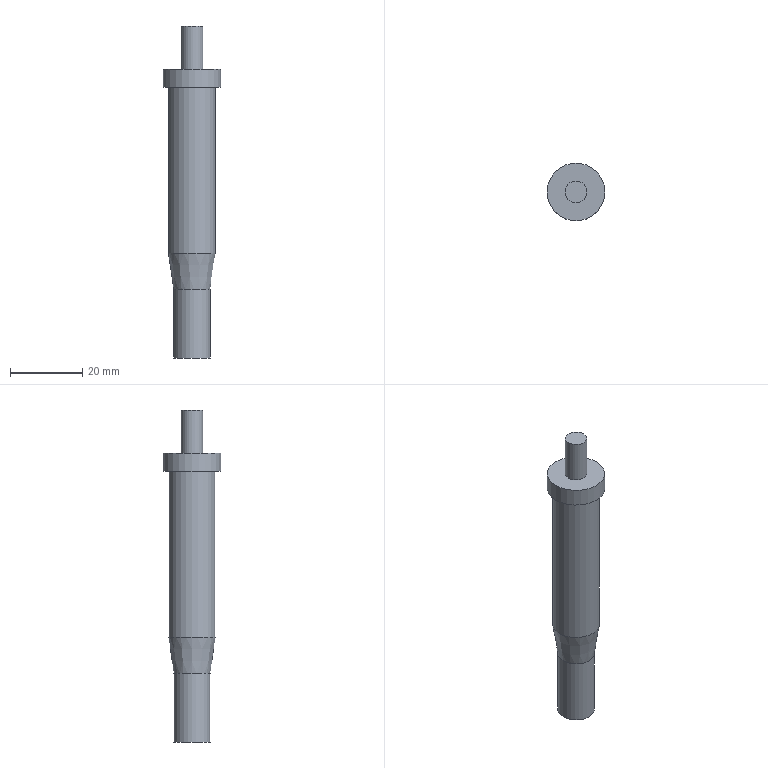Part | NX | features solid 2 | 1 solid | 9 faces | box 16 x 16 x 92 mm | volume 10026 mm3 | plane 4 | cylinder 4 | cone 1 | commonest cylinder face diameters 6 x1 10.1 x1 13 x1 16 x1
STEP:
#1=CARTESIAN_POINT('',(340.094,-150.538,50.));
#2=VERTEX_POINT('',#1);
#3=CARTESIAN_POINT('',(345.144,-150.538,50.));
#4=DIRECTION('',(0.,0.,-1.));
#5=DIRECTION('',(-1.,0.,0.));
#6=AXIS2_PLACEMENT_3D('',#3,#4,#5);
#7=CIRCLE('',#6,5.05);
#8=EDGE_CURVE('',#2,#2,#7,.T.);
#9=ORIENTED_EDGE('',*,*,#8,.T.);
#10=EDGE_LOOP('',(#9));
#11=FACE_BOUND('',#10,.T.);
#12=CARTESIAN_POINT('',(345.144,-150.538,50.));
#13=DIRECTION('',(0.,0.,-1.));
#14=DIRECTION('',(1.,0.,0.));
#15=AXIS2_PLACEMENT_3D('',#12,#13,#14);
#16=PLANE('',#15);
#17=ADVANCED_FACE('',(#11),#16,.T.);
#18=CARTESIAN_POINT('',(340.094,-150.538,69.));
#19=VERTEX_POINT('',#18);
#20=CARTESIAN_POINT('',(345.144,-150.538,69.));
#21=DIRECTION('',(0.,0.,-1.));
#22=DIRECTION('',(-1.,0.,0.));
#23=AXIS2_PLACEMENT_3D('',#20,#21,#22);
#24=CIRCLE('',#23,5.05);
#25=EDGE_CURVE('',#19,#19,#24,.T.);
#26=ORIENTED_EDGE('',*,*,#25,.T.);
#27=EDGE_LOOP('',(#26));
#28=FACE_BOUND('',#27,.T.);
#29=ORIENTED_EDGE('',*,*,#8,.F.);
#30=EDGE_LOOP('',(#29));
#31=FACE_BOUND('',#30,.T.);
#32=CARTESIAN_POINT('',(345.144,-150.538,50.));
#33=DIRECTION('',(0.,0.,1.));
#34=DIRECTION('',(-1.,0.,0.));
#35=AXIS2_PLACEMENT_3D('',#32,#33,#34);
#36=CYLINDRICAL_SURFACE('',#35,5.05);
#37=ADVANCED_FACE('',(#28,#31),#36,.T.);
#38=ORIENTED_EDGE('',*,*,#25,.F.);
#39=EDGE_LOOP('',(#38));
#40=FACE_BOUND('',#39,.T.);
#41=CARTESIAN_POINT('',(338.644,-150.538,79.));
#42=VERTEX_POINT('',#41);
#43=CARTESIAN_POINT('',(345.144,-150.538,79.));
#44=DIRECTION('',(0.,0.,-1.));
#45=DIRECTION('',(-1.,0.,0.));
#46=AXIS2_PLACEMENT_3D('',#43,#44,#45);
#47=CIRCLE('',#46,6.5);
#48=EDGE_CURVE('',#42,#42,#47,.T.);
#49=ORIENTED_EDGE('',*,*,#48,.T.);
#50=EDGE_LOOP('',(#49));
#51=FACE_BOUND('',#50,.T.);
#52=CARTESIAN_POINT('',(345.144,-150.538,69.));
#53=DIRECTION('',(0.,0.,1.));
#54=DIRECTION('',(-1.,0.,0.));
#55=AXIS2_PLACEMENT_3D('',#52,#53,#54);
#56=CONICAL_SURFACE('',#55,5.05,0.144);
#57=ADVANCED_FACE('',(#40,#51),#56,.T.);
#58=CARTESIAN_POINT('',(351.644,-150.538,125.));
#59=VERTEX_POINT('',#58);
#60=CARTESIAN_POINT('',(345.144,-150.538,125.));
#61=DIRECTION('',(0.,0.,1.));
#62=DIRECTION('',(1.,0.,0.));
#63=AXIS2_PLACEMENT_3D('',#60,#61,#62);
#64=CIRCLE('',#63,6.5);
#65=EDGE_CURVE('',#59,#59,#64,.F.);
#66=ORIENTED_EDGE('',*,*,#65,.T.);
#67=EDGE_LOOP('',(#66));
#68=FACE_BOUND('',#67,.T.);
#69=ORIENTED_EDGE('',*,*,#48,.F.);
#70=EDGE_LOOP('',(#69));
#71=FACE_BOUND('',#70,.T.);
#72=CARTESIAN_POINT('',(345.144,-150.538,79.));
#73=DIRECTION('',(0.,0.,1.));
#74=DIRECTION('',(-1.,0.,0.));
#75=AXIS2_PLACEMENT_3D('',#72,#73,#74);
#76=CYLINDRICAL_SURFACE('',#75,6.5);
#77=ADVANCED_FACE('',(#68,#71),#76,.T.);
#78=CARTESIAN_POINT('',(342.144,-150.538,130.));
#79=VERTEX_POINT('',#78);
#80=CARTESIAN_POINT('',(345.144,-150.538,130.));
#81=DIRECTION('',(0.,0.,-1.));
#82=DIRECTION('',(-1.,0.,0.));
#83=AXIS2_PLACEMENT_3D('',#80,#81,#82);
#84=CIRCLE('',#83,3.);
#85=EDGE_CURVE('',#79,#79,#84,.T.);
#86=ORIENTED_EDGE('',*,*,#85,.T.);
#87=EDGE_LOOP('',(#86));
#88=FACE_BOUND('',#87,.T.);
#89=CARTESIAN_POINT('',(353.144,-150.538,130.));
#90=VERTEX_POINT('',#89);
#91=CARTESIAN_POINT('',(345.144,-150.538,130.));
#92=DIRECTION('',(0.,0.,1.));
#93=DIRECTION('',(1.,0.,0.));
#94=AXIS2_PLACEMENT_3D('',#91,#92,#93);
#95=CIRCLE('',#94,8.);
#96=EDGE_CURVE('',#90,#90,#95,.T.);
#97=ORIENTED_EDGE('',*,*,#96,.T.);
#98=EDGE_LOOP('',(#97));
#99=FACE_BOUND('',#98,.T.);
#100=CARTESIAN_POINT('',(345.144,-150.538,130.));
#101=DIRECTION('',(0.,0.,1.));
#102=DIRECTION('',(-1.,0.,0.));
#103=AXIS2_PLACEMENT_3D('',#100,#101,#102);
#104=PLANE('',#103);
#105=ADVANCED_FACE('',(#88,#99),#104,.T.);
#106=ORIENTED_EDGE('',*,*,#65,.F.);
#107=EDGE_LOOP('',(#106));
#108=FACE_BOUND('',#107,.T.);
#109=CARTESIAN_POINT('',(337.144,-150.538,125.));
#110=VERTEX_POINT('',#109);
#111=CARTESIAN_POINT('',(345.144,-150.538,125.));
#112=DIRECTION('',(0.,0.,-1.));
#113=DIRECTION('',(-1.,0.,0.));
#114=AXIS2_PLACEMENT_3D('',#111,#112,#113);
#115=CIRCLE('',#114,8.);
#116=EDGE_CURVE('',#110,#110,#115,.T.);
#117=ORIENTED_EDGE('',*,*,#116,.T.);
#118=EDGE_LOOP('',(#117));
#119=FACE_BOUND('',#118,.T.);
#120=CARTESIAN_POINT('',(345.144,-150.538,125.));
#121=DIRECTION('',(0.,0.,-1.));
#122=DIRECTION('',(1.,0.,0.));
#123=AXIS2_PLACEMENT_3D('',#120,#121,#122);
#124=PLANE('',#123);
#125=ADVANCED_FACE('',(#108,#119),#124,.T.);
#126=ORIENTED_EDGE('',*,*,#96,.F.);
#127=EDGE_LOOP('',(#126));
#128=FACE_BOUND('',#127,.T.);
#129=ORIENTED_EDGE('',*,*,#116,.F.);
#130=EDGE_LOOP('',(#129));
#131=FACE_BOUND('',#130,.T.);
#132=CARTESIAN_POINT('',(345.144,-150.538,125.));
#133=DIRECTION('',(0.,0.,1.));
#134=DIRECTION('',(-1.,0.,0.));
#135=AXIS2_PLACEMENT_3D('',#132,#133,#134);
#136=CYLINDRICAL_SURFACE('',#135,8.);
#137=ADVANCED_FACE('',(#128,#131),#136,.T.);
#138=CARTESIAN_POINT('',(348.144,-150.538,142.));
#139=VERTEX_POINT('',#138);
#140=CARTESIAN_POINT('',(345.144,-150.538,142.));
#141=DIRECTION('',(0.,0.,1.));
#142=DIRECTION('',(1.,0.,0.));
#143=AXIS2_PLACEMENT_3D('',#140,#141,#142);
#144=CIRCLE('',#143,3.);
#145=EDGE_CURVE('',#139,#139,#144,.T.);
#146=ORIENTED_EDGE('',*,*,#145,.T.);
#147=EDGE_LOOP('',(#146));
#148=FACE_BOUND('',#147,.T.);
#149=CARTESIAN_POINT('',(345.144,-150.538,142.));
#150=DIRECTION('',(0.,0.,1.));
#151=DIRECTION('',(-1.,0.,0.));
#152=AXIS2_PLACEMENT_3D('',#149,#150,#151);
#153=PLANE('',#152);
#154=ADVANCED_FACE('',(#148),#153,.T.);
#155=ORIENTED_EDGE('',*,*,#145,.F.);
#156=EDGE_LOOP('',(#155));
#157=FACE_BOUND('',#156,.T.);
#158=ORIENTED_EDGE('',*,*,#85,.F.);
#159=EDGE_LOOP('',(#158));
#160=FACE_BOUND('',#159,.T.);
#161=CARTESIAN_POINT('',(345.144,-150.538,130.));
#162=DIRECTION('',(0.,0.,1.));
#163=DIRECTION('',(-1.,0.,0.));
#164=AXIS2_PLACEMENT_3D('',#161,#162,#163);
#165=CYLINDRICAL_SURFACE('',#164,3.);
#166=ADVANCED_FACE('',(#157,#160),#165,.T.);
#167=CLOSED_SHELL('',(#17,#37,#57,#77,#105,#125,#137,#154,#166));
#168=MANIFOLD_SOLID_BREP('',#167);
#169=(LENGTH_UNIT()NAMED_UNIT(*)SI_UNIT(.MILLI.,.METRE.));
#170=UNCERTAINTY_MEASURE_WITH_UNIT(LENGTH_MEASURE(0.00001),#169,'','');
#171=(NAMED_UNIT(*)PLANE_ANGLE_UNIT()SI_UNIT($,.RADIAN.));
#172=(NAMED_UNIT(*)SI_UNIT($,.STERADIAN.)SOLID_ANGLE_UNIT());
#173=(GEOMETRIC_REPRESENTATION_CONTEXT(3)GLOBAL_UNCERTAINTY_ASSIGNED_CONTEXT((#170))GLOBAL_UNIT_ASSIGNED_CONTEXT((#169,#171,#172))REPRESENTATION_CONTEXT('',''));
#174=ADVANCED_BREP_SHAPE_REPRESENTATION('',(#168),#173);